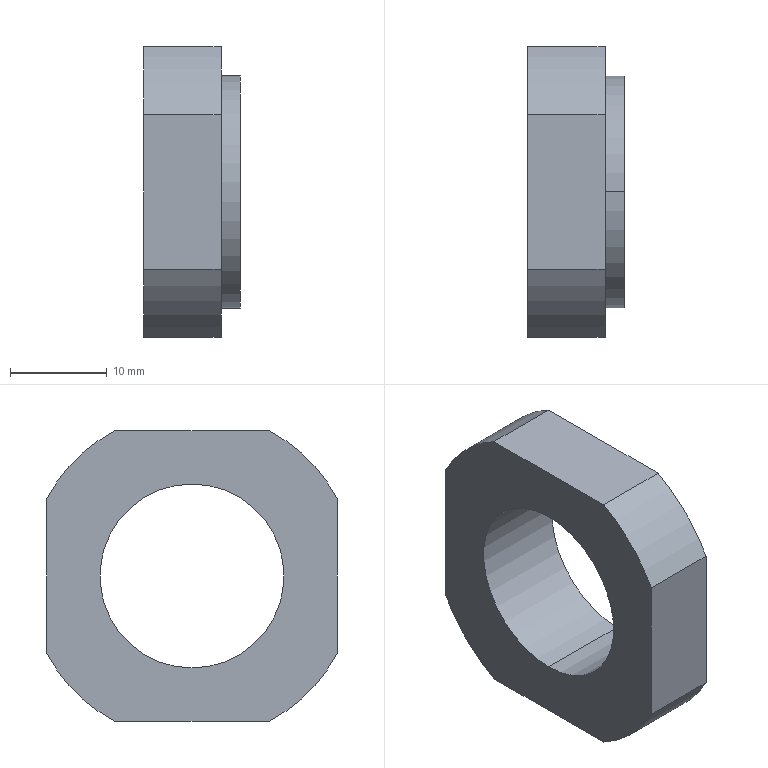Part | STEP file | PN_0006 nut | 1 solid | 15 faces | box 10 x 30 x 30 mm | volume 4642 mm3 | cylinder 8 | plane 7 | commonest cylinder face diameters 34 x4 19 x2 24 x2
STEP:
#1=CARTESIAN_POINT('',(0.,0.,0.));
#2=DIRECTION('',(0.,0.,1.));
#3=DIRECTION('',(1.,0.,0.));
#4=AXIS2_PLACEMENT_3D('',#1,#2,#3);
#5=CARTESIAN_POINT('',(-10.,0.,-9.5));
#6=VERTEX_POINT('',#5);
#7=CARTESIAN_POINT('',(0.,0.,-9.5));
#8=VERTEX_POINT('',#7);
#9=CARTESIAN_POINT('',(-10.,0.,-9.5));
#10=DIRECTION('',(1.,0.,0.));
#11=VECTOR('',#10,1.);
#12=LINE('',#9,#11);
#13=CARTESIAN_POINT('',(-10.,0.,0.));
#14=DIRECTION('',(1.,0.,0.));
#15=DIRECTION('',(0.,0.,-1.));
#16=AXIS2_PLACEMENT_3D('',#13,#14,#15);
#17=CYLINDRICAL_SURFACE('',#16,9.5);
#18=CARTESIAN_POINT('',(6.283,0.));
#19=DIRECTION('',(0.,1.));
#20=VECTOR('',#19,1.);
#21=LINE('',#18,#20);
#22=(GEOMETRIC_REPRESENTATION_CONTEXT(2)PARAMETRIC_REPRESENTATION_CONTEXT()REPRESENTATION_CONTEXT('',''));
#23=DEFINITIONAL_REPRESENTATION('',(#21),#22);
#24=PCURVE('',#17,#23);
#25=CARTESIAN_POINT('',(-10.,0.,0.));
#26=DIRECTION('',(1.,0.,0.));
#27=DIRECTION('',(0.,0.,-1.));
#28=AXIS2_PLACEMENT_3D('',#25,#26,#27);
#29=CYLINDRICAL_SURFACE('',#28,9.5);
#30=CARTESIAN_POINT('',(0.,0.));
#31=DIRECTION('',(0.,1.));
#32=VECTOR('',#31,1.);
#33=LINE('',#30,#32);
#34=(GEOMETRIC_REPRESENTATION_CONTEXT(2)PARAMETRIC_REPRESENTATION_CONTEXT()REPRESENTATION_CONTEXT('',''));
#35=DEFINITIONAL_REPRESENTATION('',(#33),#34);
#36=PCURVE('',#29,#35);
#37=SURFACE_CURVE('',#12,(#24,#36),.PCURVE_S1.);
#38=EDGE_CURVE('',#6,#8,#37,.T.);
#39=ORIENTED_EDGE('',*,*,#38,.T.);
#40=CARTESIAN_POINT('',(0.,0.,9.5));
#41=VERTEX_POINT('',#40);
#42=CARTESIAN_POINT('',(0.,0.,0.));
#43=DIRECTION('',(1.,0.,0.));
#44=DIRECTION('',(0.,0.,-1.));
#45=AXIS2_PLACEMENT_3D('',#42,#43,#44);
#46=CIRCLE('',#45,9.5);
#47=CARTESIAN_POINT('',(0.,10.));
#48=DIRECTION('',(1.,0.));
#49=VECTOR('',#48,1.);
#50=LINE('',#47,#49);
#51=(GEOMETRIC_REPRESENTATION_CONTEXT(2)PARAMETRIC_REPRESENTATION_CONTEXT()REPRESENTATION_CONTEXT('',''));
#52=DEFINITIONAL_REPRESENTATION('',(#50),#51);
#53=PCURVE('',#17,#52);
#54=CARTESIAN_POINT('',(0.,0.,0.));
#55=DIRECTION('',(1.,0.,0.));
#56=DIRECTION('',(0.,0.,-1.));
#57=AXIS2_PLACEMENT_3D('',#54,#55,#56);
#58=PLANE('',#57);
#59=CARTESIAN_POINT('',(0.,0.));
#60=DIRECTION('',(1.,0.));
#61=AXIS2_PLACEMENT_2D('',#59,#60);
#62=CIRCLE('',#61,9.5);
#63=(GEOMETRIC_REPRESENTATION_CONTEXT(2)PARAMETRIC_REPRESENTATION_CONTEXT()REPRESENTATION_CONTEXT('',''));
#64=DEFINITIONAL_REPRESENTATION('',(#62),#63);
#65=PCURVE('',#58,#64);
#66=SURFACE_CURVE('',#46,(#53,#65),.PCURVE_S1.);
#67=EDGE_CURVE('',#41,#8,#66,.T.);
#68=ORIENTED_EDGE('',*,*,#67,.F.);
#69=CARTESIAN_POINT('',(-10.,0.,9.5));
#70=VERTEX_POINT('',#69);
#71=CARTESIAN_POINT('',(-10.,0.,9.5));
#72=DIRECTION('',(1.,0.,0.));
#73=VECTOR('',#72,1.);
#74=LINE('',#71,#73);
#75=CARTESIAN_POINT('',(3.142,0.));
#76=DIRECTION('',(0.,1.));
#77=VECTOR('',#76,1.);
#78=LINE('',#75,#77);
#79=(GEOMETRIC_REPRESENTATION_CONTEXT(2)PARAMETRIC_REPRESENTATION_CONTEXT()REPRESENTATION_CONTEXT('',''));
#80=DEFINITIONAL_REPRESENTATION('',(#78),#79);
#81=PCURVE('',#17,#80);
#82=CARTESIAN_POINT('',(3.142,0.));
#83=DIRECTION('',(0.,1.));
#84=VECTOR('',#83,1.);
#85=LINE('',#82,#84);
#86=(GEOMETRIC_REPRESENTATION_CONTEXT(2)PARAMETRIC_REPRESENTATION_CONTEXT()REPRESENTATION_CONTEXT('',''));
#87=DEFINITIONAL_REPRESENTATION('',(#85),#86);
#88=PCURVE('',#29,#87);
#89=SURFACE_CURVE('',#74,(#81,#88),.PCURVE_S1.);
#90=EDGE_CURVE('',#70,#41,#89,.T.);
#91=ORIENTED_EDGE('',*,*,#90,.F.);
#92=CARTESIAN_POINT('',(-10.,0.,0.));
#93=DIRECTION('',(1.,0.,0.));
#94=DIRECTION('',(0.,0.,-1.));
#95=AXIS2_PLACEMENT_3D('',#92,#93,#94);
#96=CIRCLE('',#95,9.5);
#97=CARTESIAN_POINT('',(0.,0.));
#98=DIRECTION('',(1.,0.));
#99=VECTOR('',#98,1.);
#100=LINE('',#97,#99);
#101=(GEOMETRIC_REPRESENTATION_CONTEXT(2)PARAMETRIC_REPRESENTATION_CONTEXT()REPRESENTATION_CONTEXT('',''));
#102=DEFINITIONAL_REPRESENTATION('',(#100),#101);
#103=PCURVE('',#17,#102);
#104=CARTESIAN_POINT('',(-10.,17.,0.));
#105=DIRECTION('',(-1.,0.,0.));
#106=DIRECTION('',(0.,0.,1.));
#107=AXIS2_PLACEMENT_3D('',#104,#105,#106);
#108=PLANE('',#107);
#109=CARTESIAN_POINT('',(-9.5,-17.));
#110=CARTESIAN_POINT('',(-9.5,-0.5455));
#111=CARTESIAN_POINT('',(4.75,-8.773));
#112=CARTESIAN_POINT('',(19.,-17.));
#113=CARTESIAN_POINT('',(4.75,-25.227));
#114=CARTESIAN_POINT('',(-9.5,-33.454));
#115=CARTESIAN_POINT('',(-9.5,-17.));
#116=(BOUNDED_CURVE()B_SPLINE_CURVE(2,(#109,#110,#111,#112,#113,#114,#115),.UNSPECIFIED.,.T.,.F.)B_SPLINE_CURVE_WITH_KNOTS((1,2,2,2,2,1),(-2.094,0.,2.094,4.189,6.283,8.378),.UNSPECIFIED.)CURVE()GEOMETRIC_REPRESENTATION_ITEM()RATIONAL_B_SPLINE_CURVE((1.,0.5,1.,0.5,1.,0.5,1.))REPRESENTATION_ITEM(''));
#117=(GEOMETRIC_REPRESENTATION_CONTEXT(2)PARAMETRIC_REPRESENTATION_CONTEXT()REPRESENTATION_CONTEXT('',''));
#118=DEFINITIONAL_REPRESENTATION('',(#116),#117);
#119=PCURVE('',#108,#118);
#120=SURFACE_CURVE('',#96,(#103,#119),.PCURVE_S1.);
#121=EDGE_CURVE('',#70,#6,#120,.T.);
#122=ORIENTED_EDGE('',*,*,#121,.T.);
#123=EDGE_LOOP('',(#39,#68,#91,#122));
#124=FACE_BOUND('',#123,.F.);
#125=ADVANCED_FACE('',(#124),#17,.F.);
#126=CARTESIAN_POINT('',(-2.,0.,-12.));
#127=VERTEX_POINT('',#126);
#128=CARTESIAN_POINT('',(-2.,0.,12.));
#129=VERTEX_POINT('',#128);
#130=CARTESIAN_POINT('',(-2.,0.,0.));
#131=DIRECTION('',(1.,0.,0.));
#132=DIRECTION('',(0.,0.,-1.));
#133=AXIS2_PLACEMENT_3D('',#130,#131,#132);
#134=CIRCLE('',#133,12.);
#135=CARTESIAN_POINT('',(0.,0.,0.));
#136=DIRECTION('',(1.,0.,0.));
#137=DIRECTION('',(0.,0.,-1.));
#138=AXIS2_PLACEMENT_3D('',#135,#136,#137);
#139=CYLINDRICAL_SURFACE('',#138,12.);
#140=CARTESIAN_POINT('',(0.,-2.));
#141=DIRECTION('',(1.,0.));
#142=VECTOR('',#141,1.);
#143=LINE('',#140,#142);
#144=(GEOMETRIC_REPRESENTATION_CONTEXT(2)PARAMETRIC_REPRESENTATION_CONTEXT()REPRESENTATION_CONTEXT('',''));
#145=DEFINITIONAL_REPRESENTATION('',(#143),#144);
#146=PCURVE('',#139,#145);
#147=CARTESIAN_POINT('',(-2.,12.,0.));
#148=DIRECTION('',(1.,0.,0.));
#149=DIRECTION('',(0.,0.,-1.));
#150=AXIS2_PLACEMENT_3D('',#147,#148,#149);
#151=PLANE('',#150);
#152=CARTESIAN_POINT('',(0.,-12.));
#153=DIRECTION('',(1.,0.));
#154=AXIS2_PLACEMENT_2D('',#152,#153);
#155=CIRCLE('',#154,12.);
#156=(GEOMETRIC_REPRESENTATION_CONTEXT(2)PARAMETRIC_REPRESENTATION_CONTEXT()REPRESENTATION_CONTEXT('',''));
#157=DEFINITIONAL_REPRESENTATION('',(#155),#156);
#158=PCURVE('',#151,#157);
#159=SURFACE_CURVE('',#134,(#146,#158),.PCURVE_S1.);
#160=EDGE_CURVE('',#127,#129,#159,.T.);
#161=ORIENTED_EDGE('',*,*,#160,.T.);
#162=CARTESIAN_POINT('',(0.,0.,12.));
#163=VERTEX_POINT('',#162);
#164=CARTESIAN_POINT('',(0.,0.,12.));
#165=DIRECTION('',(1.,0.,0.));
#166=VECTOR('',#165,1.);
#167=LINE('',#164,#166);
#168=CARTESIAN_POINT('',(3.142,0.));
#169=DIRECTION('',(0.,1.));
#170=VECTOR('',#169,1.);
#171=LINE('',#168,#170);
#172=(GEOMETRIC_REPRESENTATION_CONTEXT(2)PARAMETRIC_REPRESENTATION_CONTEXT()REPRESENTATION_CONTEXT('',''));
#173=DEFINITIONAL_REPRESENTATION('',(#171),#172);
#174=PCURVE('',#139,#173);
#175=CARTESIAN_POINT('',(0.,0.,0.));
#176=DIRECTION('',(1.,0.,0.));
#177=DIRECTION('',(0.,0.,-1.));
#178=AXIS2_PLACEMENT_3D('',#175,#176,#177);
#179=CYLINDRICAL_SURFACE('',#178,12.);
#180=CARTESIAN_POINT('',(3.142,0.));
#181=DIRECTION('',(0.,1.));
#182=VECTOR('',#181,1.);
#183=LINE('',#180,#182);
#184=(GEOMETRIC_REPRESENTATION_CONTEXT(2)PARAMETRIC_REPRESENTATION_CONTEXT()REPRESENTATION_CONTEXT('',''));
#185=DEFINITIONAL_REPRESENTATION('',(#183),#184);
#186=PCURVE('',#179,#185);
#187=SURFACE_CURVE('',#167,(#174,#186),.PCURVE_S1.);
#188=EDGE_CURVE('',#129,#163,#187,.T.);
#189=ORIENTED_EDGE('',*,*,#188,.T.);
#190=CARTESIAN_POINT('',(0.,0.,-12.));
#191=VERTEX_POINT('',#190);
#192=CARTESIAN_POINT('',(0.,0.,0.));
#193=DIRECTION('',(1.,0.,0.));
#194=DIRECTION('',(0.,0.,-1.));
#195=AXIS2_PLACEMENT_3D('',#192,#193,#194);
#196=CIRCLE('',#195,12.);
#197=CARTESIAN_POINT('',(0.,0.));
#198=DIRECTION('',(1.,0.));
#199=VECTOR('',#198,1.);
#200=LINE('',#197,#199);
#201=(GEOMETRIC_REPRESENTATION_CONTEXT(2)PARAMETRIC_REPRESENTATION_CONTEXT()REPRESENTATION_CONTEXT('',''));
#202=DEFINITIONAL_REPRESENTATION('',(#200),#201);
#203=PCURVE('',#139,#202);
#204=CARTESIAN_POINT('',(0.,0.));
#205=DIRECTION('',(1.,0.));
#206=AXIS2_PLACEMENT_2D('',#204,#205);
#207=CIRCLE('',#206,12.);
#208=(GEOMETRIC_REPRESENTATION_CONTEXT(2)PARAMETRIC_REPRESENTATION_CONTEXT()REPRESENTATION_CONTEXT('',''));
#209=DEFINITIONAL_REPRESENTATION('',(#207),#208);
#210=PCURVE('',#58,#209);
#211=SURFACE_CURVE('',#196,(#203,#210),.PCURVE_S1.);
#212=EDGE_CURVE('',#191,#163,#211,.T.);
#213=ORIENTED_EDGE('',*,*,#212,.F.);
#214=CARTESIAN_POINT('',(0.,0.,-12.));
#215=DIRECTION('',(1.,0.,0.));
#216=VECTOR('',#215,1.);
#217=LINE('',#214,#216);
#218=CARTESIAN_POINT('',(0.,0.));
#219=DIRECTION('',(0.,1.));
#220=VECTOR('',#219,1.);
#221=LINE('',#218,#220);
#222=(GEOMETRIC_REPRESENTATION_CONTEXT(2)PARAMETRIC_REPRESENTATION_CONTEXT()REPRESENTATION_CONTEXT('',''));
#223=DEFINITIONAL_REPRESENTATION('',(#221),#222);
#224=PCURVE('',#139,#223);
#225=CARTESIAN_POINT('',(6.283,0.));
#226=DIRECTION('',(0.,1.));
#227=VECTOR('',#226,1.);
#228=LINE('',#225,#227);
#229=(GEOMETRIC_REPRESENTATION_CONTEXT(2)PARAMETRIC_REPRESENTATION_CONTEXT()REPRESENTATION_CONTEXT('',''));
#230=DEFINITIONAL_REPRESENTATION('',(#228),#229);
#231=PCURVE('',#179,#230);
#232=SURFACE_CURVE('',#217,(#224,#231),.PCURVE_S1.);
#233=EDGE_CURVE('',#127,#191,#232,.T.);
#234=ORIENTED_EDGE('',*,*,#233,.F.);
#235=EDGE_LOOP('',(#161,#189,#213,#234));
#236=FACE_BOUND('',#235,.T.);
#237=ADVANCED_FACE('',(#236),#139,.T.);
#238=CARTESIAN_POINT('',(-2.,8.,15.));
#239=VERTEX_POINT('',#238);
#240=CARTESIAN_POINT('',(-10.,8.,15.));
#241=VERTEX_POINT('',#240);
#242=CARTESIAN_POINT('',(0.,8.,15.));
#243=DIRECTION('',(-1.,0.,0.));
#244=VECTOR('',#243,1.);
#245=LINE('',#242,#244);
#246=CARTESIAN_POINT('',(0.,0.,0.));
#247=DIRECTION('',(1.,0.,0.));
#248=DIRECTION('',(0.,0.,-1.));
#249=AXIS2_PLACEMENT_3D('',#246,#247,#248);
#250=CYLINDRICAL_SURFACE('',#249,17.);
#251=CARTESIAN_POINT('',(2.652,0.));
#252=DIRECTION('',(0.,-1.));
#253=VECTOR('',#252,1.);
#254=LINE('',#251,#253);
#255=(GEOMETRIC_REPRESENTATION_CONTEXT(2)PARAMETRIC_REPRESENTATION_CONTEXT()REPRESENTATION_CONTEXT('',''));
#256=DEFINITIONAL_REPRESENTATION('',(#254),#255);
#257=PCURVE('',#250,#256);
#258=CARTESIAN_POINT('',(0.,17.205,15.));
#259=DIRECTION('',(0.,0.,-1.));
#260=DIRECTION('',(0.,1.,0.));
#261=AXIS2_PLACEMENT_3D('',#258,#259,#260);
#262=PLANE('',#261);
#263=CARTESIAN_POINT('',(-9.205,0.));
#264=DIRECTION('',(0.,-1.));
#265=VECTOR('',#264,1.);
#266=LINE('',#263,#265);
#267=(GEOMETRIC_REPRESENTATION_CONTEXT(2)PARAMETRIC_REPRESENTATION_CONTEXT()REPRESENTATION_CONTEXT('',''));
#268=DEFINITIONAL_REPRESENTATION('',(#266),#267);
#269=PCURVE('',#262,#268);
#270=SURFACE_CURVE('',#245,(#257,#269),.PCURVE_S1.);
#271=EDGE_CURVE('',#239,#241,#270,.T.);
#272=ORIENTED_EDGE('',*,*,#271,.F.);
#273=CARTESIAN_POINT('',(-2.,15.,8.));
#274=VERTEX_POINT('',#273);
#275=CARTESIAN_POINT('',(-2.,0.,0.));
#276=DIRECTION('',(1.,0.,0.));
#277=DIRECTION('',(0.,0.,-1.));
#278=AXIS2_PLACEMENT_3D('',#275,#276,#277);
#279=CIRCLE('',#278,17.);
#280=CARTESIAN_POINT('',(0.,-2.));
#281=DIRECTION('',(1.,0.));
#282=VECTOR('',#281,1.);
#283=LINE('',#280,#282);
#284=(GEOMETRIC_REPRESENTATION_CONTEXT(2)PARAMETRIC_REPRESENTATION_CONTEXT()REPRESENTATION_CONTEXT('',''));
#285=DEFINITIONAL_REPRESENTATION('',(#283),#284);
#286=PCURVE('',#250,#285);
#287=CARTESIAN_POINT('',(0.,-12.));
#288=DIRECTION('',(1.,0.));
#289=AXIS2_PLACEMENT_2D('',#287,#288);
#290=CIRCLE('',#289,17.);
#291=(GEOMETRIC_REPRESENTATION_CONTEXT(2)PARAMETRIC_REPRESENTATION_CONTEXT()REPRESENTATION_CONTEXT('',''));
#292=DEFINITIONAL_REPRESENTATION('',(#290),#291);
#293=PCURVE('',#151,#292);
#294=SURFACE_CURVE('',#279,(#286,#293),.PCURVE_S1.);
#295=EDGE_CURVE('',#274,#239,#294,.T.);
#296=ORIENTED_EDGE('',*,*,#295,.F.);
#297=CARTESIAN_POINT('',(-10.,15.,8.));
#298=VERTEX_POINT('',#297);
#299=CARTESIAN_POINT('',(0.,15.,8.));
#300=DIRECTION('',(1.,0.,0.));
#301=VECTOR('',#300,1.);
#302=LINE('',#299,#301);
#303=CARTESIAN_POINT('',(2.061,0.));
#304=DIRECTION('',(0.,1.));
#305=VECTOR('',#304,1.);
#306=LINE('',#303,#305);
#307=(GEOMETRIC_REPRESENTATION_CONTEXT(2)PARAMETRIC_REPRESENTATION_CONTEXT()REPRESENTATION_CONTEXT('',''));
#308=DEFINITIONAL_REPRESENTATION('',(#306),#307);
#309=PCURVE('',#250,#308);
#310=CARTESIAN_POINT('',(0.,15.,-20.296));
#311=DIRECTION('',(0.,-1.,0.));
#312=DIRECTION('',(0.,0.,-1.));
#313=AXIS2_PLACEMENT_3D('',#310,#311,#312);
#314=PLANE('',#313);
#315=CARTESIAN_POINT('',(-28.296,0.));
#316=DIRECTION('',(0.,1.));
#317=VECTOR('',#316,1.);
#318=LINE('',#315,#317);
#319=(GEOMETRIC_REPRESENTATION_CONTEXT(2)PARAMETRIC_REPRESENTATION_CONTEXT()REPRESENTATION_CONTEXT('',''));
#320=DEFINITIONAL_REPRESENTATION('',(#318),#319);
#321=PCURVE('',#314,#320);
#322=SURFACE_CURVE('',#302,(#309,#321),.PCURVE_S1.);
#323=EDGE_CURVE('',#298,#274,#322,.T.);
#324=ORIENTED_EDGE('',*,*,#323,.F.);
#325=CARTESIAN_POINT('',(-10.,0.,0.));
#326=DIRECTION('',(1.,0.,0.));
#327=DIRECTION('',(0.,0.,-1.));
#328=AXIS2_PLACEMENT_3D('',#325,#326,#327);
#329=CIRCLE('',#328,17.);
#330=CARTESIAN_POINT('',(0.,-10.));
#331=DIRECTION('',(1.,0.));
#332=VECTOR('',#331,1.);
#333=LINE('',#330,#332);
#334=(GEOMETRIC_REPRESENTATION_CONTEXT(2)PARAMETRIC_REPRESENTATION_CONTEXT()REPRESENTATION_CONTEXT('',''));
#335=DEFINITIONAL_REPRESENTATION('',(#333),#334);
#336=PCURVE('',#250,#335);
#337=CARTESIAN_POINT('',(-17.,-17.));
#338=CARTESIAN_POINT('',(-17.,12.445));
#339=CARTESIAN_POINT('',(8.5,-2.278));
#340=CARTESIAN_POINT('',(34.,-17.));
#341=CARTESIAN_POINT('',(8.5,-31.722));
#342=CARTESIAN_POINT('',(-17.,-46.445));
#343=CARTESIAN_POINT('',(-17.,-17.));
#344=(BOUNDED_CURVE()B_SPLINE_CURVE(2,(#337,#338,#339,#340,#341,#342,#343),.UNSPECIFIED.,.T.,.F.)B_SPLINE_CURVE_WITH_KNOTS((1,2,2,2,2,1),(-2.094,0.,2.094,4.189,6.283,8.378),.UNSPECIFIED.)CURVE()GEOMETRIC_REPRESENTATION_ITEM()RATIONAL_B_SPLINE_CURVE((1.,0.5,1.,0.5,1.,0.5,1.))REPRESENTATION_ITEM(''));
#345=(GEOMETRIC_REPRESENTATION_CONTEXT(2)PARAMETRIC_REPRESENTATION_CONTEXT()REPRESENTATION_CONTEXT('',''));
#346=DEFINITIONAL_REPRESENTATION('',(#344),#345);
#347=PCURVE('',#108,#346);
#348=SURFACE_CURVE('',#329,(#336,#347),.PCURVE_S1.);
#349=EDGE_CURVE('',#298,#241,#348,.T.);
#350=ORIENTED_EDGE('',*,*,#349,.T.);
#351=EDGE_LOOP('',(#272,#296,#324,#350));
#352=FACE_BOUND('',#351,.T.);
#353=ADVANCED_FACE('',(#352),#250,.T.);
#354=CARTESIAN_POINT('',(-2.,-8.,-15.));
#355=VERTEX_POINT('',#354);
#356=CARTESIAN_POINT('',(-10.,-8.,-15.));
#357=VERTEX_POINT('',#356);
#358=CARTESIAN_POINT('',(0.,-8.,-15.));
#359=DIRECTION('',(-1.,0.,0.));
#360=VECTOR('',#359,1.);
#361=LINE('',#358,#360);
#362=CARTESIAN_POINT('',(0.,0.,0.));
#363=DIRECTION('',(1.,0.,0.));
#364=DIRECTION('',(0.,0.,-1.));
#365=AXIS2_PLACEMENT_3D('',#362,#363,#364);
#366=CYLINDRICAL_SURFACE('',#365,17.);
#367=CARTESIAN_POINT('',(5.793,0.));
#368=DIRECTION('',(0.,-1.));
#369=VECTOR('',#368,1.);
#370=LINE('',#367,#369);
#371=(GEOMETRIC_REPRESENTATION_CONTEXT(2)PARAMETRIC_REPRESENTATION_CONTEXT()REPRESENTATION_CONTEXT('',''));
#372=DEFINITIONAL_REPRESENTATION('',(#370),#371);
#373=PCURVE('',#366,#372);
#374=CARTESIAN_POINT('',(0.,17.205,-15.));
#375=DIRECTION('',(0.,0.,1.));
#376=DIRECTION('',(0.,-1.,0.));
#377=AXIS2_PLACEMENT_3D('',#374,#375,#376);
#378=PLANE('',#377);
#379=CARTESIAN_POINT('',(25.205,0.));
#380=DIRECTION('',(0.,-1.));
#381=VECTOR('',#380,1.);
#382=LINE('',#379,#381);
#383=(GEOMETRIC_REPRESENTATION_CONTEXT(2)PARAMETRIC_REPRESENTATION_CONTEXT()REPRESENTATION_CONTEXT('',''));
#384=DEFINITIONAL_REPRESENTATION('',(#382),#383);
#385=PCURVE('',#378,#384);
#386=SURFACE_CURVE('',#361,(#373,#385),.PCURVE_S1.);
#387=EDGE_CURVE('',#355,#357,#386,.T.);
#388=ORIENTED_EDGE('',*,*,#387,.F.);
#389=CARTESIAN_POINT('',(-2.,-15.,-8.));
#390=VERTEX_POINT('',#389);
#391=CARTESIAN_POINT('',(-2.,0.,0.));
#392=DIRECTION('',(1.,0.,0.));
#393=DIRECTION('',(0.,0.,-1.));
#394=AXIS2_PLACEMENT_3D('',#391,#392,#393);
#395=CIRCLE('',#394,17.);
#396=CARTESIAN_POINT('',(0.,-2.));
#397=DIRECTION('',(1.,0.));
#398=VECTOR('',#397,1.);
#399=LINE('',#396,#398);
#400=(GEOMETRIC_REPRESENTATION_CONTEXT(2)PARAMETRIC_REPRESENTATION_CONTEXT()REPRESENTATION_CONTEXT('',''));
#401=DEFINITIONAL_REPRESENTATION('',(#399),#400);
#402=PCURVE('',#366,#401);
#403=CARTESIAN_POINT('',(0.,-12.));
#404=DIRECTION('',(1.,0.));
#405=AXIS2_PLACEMENT_2D('',#403,#404);
#406=CIRCLE('',#405,17.);
#407=(GEOMETRIC_REPRESENTATION_CONTEXT(2)PARAMETRIC_REPRESENTATION_CONTEXT()REPRESENTATION_CONTEXT('',''));
#408=DEFINITIONAL_REPRESENTATION('',(#406),#407);
#409=PCURVE('',#151,#408);
#410=SURFACE_CURVE('',#395,(#402,#409),.PCURVE_S1.);
#411=EDGE_CURVE('',#390,#355,#410,.T.);
#412=ORIENTED_EDGE('',*,*,#411,.F.);
#413=CARTESIAN_POINT('',(-10.,-15.,-8.));
#414=VERTEX_POINT('',#413);
#415=CARTESIAN_POINT('',(0.,-15.,-8.));
#416=DIRECTION('',(1.,0.,0.));
#417=VECTOR('',#416,1.);
#418=LINE('',#415,#417);
#419=CARTESIAN_POINT('',(5.202,0.));
#420=DIRECTION('',(0.,1.));
#421=VECTOR('',#420,1.);
#422=LINE('',#419,#421);
#423=(GEOMETRIC_REPRESENTATION_CONTEXT(2)PARAMETRIC_REPRESENTATION_CONTEXT()REPRESENTATION_CONTEXT('',''));
#424=DEFINITIONAL_REPRESENTATION('',(#422),#423);
#425=PCURVE('',#366,#424);
#426=CARTESIAN_POINT('',(0.,-15.,-20.296));
#427=DIRECTION('',(0.,1.,0.));
#428=DIRECTION('',(0.,0.,1.));
#429=AXIS2_PLACEMENT_3D('',#426,#427,#428);
#430=PLANE('',#429);
#431=CARTESIAN_POINT('',(12.296,0.));
#432=DIRECTION('',(0.,1.));
#433=VECTOR('',#432,1.);
#434=LINE('',#431,#433);
#435=(GEOMETRIC_REPRESENTATION_CONTEXT(2)PARAMETRIC_REPRESENTATION_CONTEXT()REPRESENTATION_CONTEXT('',''));
#436=DEFINITIONAL_REPRESENTATION('',(#434),#435);
#437=PCURVE('',#430,#436);
#438=SURFACE_CURVE('',#418,(#425,#437),.PCURVE_S1.);
#439=EDGE_CURVE('',#414,#390,#438,.T.);
#440=ORIENTED_EDGE('',*,*,#439,.F.);
#441=CARTESIAN_POINT('',(-10.,0.,0.));
#442=DIRECTION('',(1.,0.,0.));
#443=DIRECTION('',(0.,0.,-1.));
#444=AXIS2_PLACEMENT_3D('',#441,#442,#443);
#445=CIRCLE('',#444,17.);
#446=CARTESIAN_POINT('',(0.,-10.));
#447=DIRECTION('',(1.,0.));
#448=VECTOR('',#447,1.);
#449=LINE('',#446,#448);
#450=(GEOMETRIC_REPRESENTATION_CONTEXT(2)PARAMETRIC_REPRESENTATION_CONTEXT()REPRESENTATION_CONTEXT('',''));
#451=DEFINITIONAL_REPRESENTATION('',(#449),#450);
#452=PCURVE('',#366,#451);
#453=CARTESIAN_POINT('',(-17.,-17.));
#454=CARTESIAN_POINT('',(-17.,12.445));
#455=CARTESIAN_POINT('',(8.5,-2.278));
#456=CARTESIAN_POINT('',(34.,-17.));
#457=CARTESIAN_POINT('',(8.5,-31.722));
#458=CARTESIAN_POINT('',(-17.,-46.445));
#459=CARTESIAN_POINT('',(-17.,-17.));
#460=(BOUNDED_CURVE()B_SPLINE_CURVE(2,(#453,#454,#455,#456,#457,#458,#459),.UNSPECIFIED.,.T.,.F.)B_SPLINE_CURVE_WITH_KNOTS((1,2,2,2,2,1),(-2.094,0.,2.094,4.189,6.283,8.378),.UNSPECIFIED.)CURVE()GEOMETRIC_REPRESENTATION_ITEM()RATIONAL_B_SPLINE_CURVE((1.,0.5,1.,0.5,1.,0.5,1.))REPRESENTATION_ITEM(''));
#461=(GEOMETRIC_REPRESENTATION_CONTEXT(2)PARAMETRIC_REPRESENTATION_CONTEXT()REPRESENTATION_CONTEXT('',''));
#462=DEFINITIONAL_REPRESENTATION('',(#460),#461);
#463=PCURVE('',#108,#462);
#464=SURFACE_CURVE('',#445,(#452,#463),.PCURVE_S1.);
#465=EDGE_CURVE('',#414,#357,#464,.T.);
#466=ORIENTED_EDGE('',*,*,#465,.T.);
#467=EDGE_LOOP('',(#388,#412,#440,#466));
#468=FACE_BOUND('',#467,.T.);
#469=ADVANCED_FACE('',(#468),#366,.T.);
#470=CARTESIAN_POINT('',(-10.,-8.,15.));
#471=VERTEX_POINT('',#470);
#472=CARTESIAN_POINT('',(-2.,-8.,15.));
#473=VERTEX_POINT('',#472);
#474=CARTESIAN_POINT('',(0.,-8.,15.));
#475=DIRECTION('',(1.,0.,0.));
#476=VECTOR('',#475,1.);
#477=LINE('',#474,#476);
#478=CARTESIAN_POINT('',(0.,0.,0.));
#479=DIRECTION('',(1.,0.,0.));
#480=DIRECTION('',(0.,0.,-1.));
#481=AXIS2_PLACEMENT_3D('',#478,#479,#480);
#482=CYLINDRICAL_SURFACE('',#481,17.);
#483=CARTESIAN_POINT('',(3.632,0.));
#484=DIRECTION('',(0.,1.));
#485=VECTOR('',#484,1.);
#486=LINE('',#483,#485);
#487=(GEOMETRIC_REPRESENTATION_CONTEXT(2)PARAMETRIC_REPRESENTATION_CONTEXT()REPRESENTATION_CONTEXT('',''));
#488=DEFINITIONAL_REPRESENTATION('',(#486),#487);
#489=PCURVE('',#482,#488);
#490=CARTESIAN_POINT('',(-25.205,0.));
#491=DIRECTION('',(0.,1.));
#492=VECTOR('',#491,1.);
#493=LINE('',#490,#492);
#494=(GEOMETRIC_REPRESENTATION_CONTEXT(2)PARAMETRIC_REPRESENTATION_CONTEXT()REPRESENTATION_CONTEXT('',''));
#495=DEFINITIONAL_REPRESENTATION('',(#493),#494);
#496=PCURVE('',#262,#495);
#497=SURFACE_CURVE('',#477,(#489,#496),.PCURVE_S1.);
#498=EDGE_CURVE('',#471,#473,#497,.T.);
#499=ORIENTED_EDGE('',*,*,#498,.F.);
#500=CARTESIAN_POINT('',(-10.,-15.,8.));
#501=VERTEX_POINT('',#500);
#502=CARTESIAN_POINT('',(-10.,0.,0.));
#503=DIRECTION('',(1.,0.,0.));
#504=DIRECTION('',(0.,0.,-1.));
#505=AXIS2_PLACEMENT_3D('',#502,#503,#504);
#506=CIRCLE('',#505,17.);
#507=CARTESIAN_POINT('',(0.,-10.));
#508=DIRECTION('',(1.,0.));
#509=VECTOR('',#508,1.);
#510=LINE('',#507,#509);
#511=(GEOMETRIC_REPRESENTATION_CONTEXT(2)PARAMETRIC_REPRESENTATION_CONTEXT()REPRESENTATION_CONTEXT('',''));
#512=DEFINITIONAL_REPRESENTATION('',(#510),#511);
#513=PCURVE('',#482,#512);
#514=CARTESIAN_POINT('',(-17.,-17.));
#515=CARTESIAN_POINT('',(-17.,12.445));
#516=CARTESIAN_POINT('',(8.5,-2.278));
#517=CARTESIAN_POINT('',(34.,-17.));
#518=CARTESIAN_POINT('',(8.5,-31.722));
#519=CARTESIAN_POINT('',(-17.,-46.445));
#520=CARTESIAN_POINT('',(-17.,-17.));
#521=(BOUNDED_CURVE()B_SPLINE_CURVE(2,(#514,#515,#516,#517,#518,#519,#520),.UNSPECIFIED.,.T.,.F.)B_SPLINE_CURVE_WITH_KNOTS((1,2,2,2,2,1),(-2.094,0.,2.094,4.189,6.283,8.378),.UNSPECIFIED.)CURVE()GEOMETRIC_REPRESENTATION_ITEM()RATIONAL_B_SPLINE_CURVE((1.,0.5,1.,0.5,1.,0.5,1.))REPRESENTATION_ITEM(''));
#522=(GEOMETRIC_REPRESENTATION_CONTEXT(2)PARAMETRIC_REPRESENTATION_CONTEXT()REPRESENTATION_CONTEXT('',''));
#523=DEFINITIONAL_REPRESENTATION('',(#521),#522);
#524=PCURVE('',#108,#523);
#525=SURFACE_CURVE('',#506,(#513,#524),.PCURVE_S1.);
#526=EDGE_CURVE('',#471,#501,#525,.T.);
#527=ORIENTED_EDGE('',*,*,#526,.T.);
#528=CARTESIAN_POINT('',(-2.,-15.,8.));
#529=VERTEX_POINT('',#528);
#530=CARTESIAN_POINT('',(0.,-15.,8.));
#531=DIRECTION('',(-1.,0.,0.));
#532=VECTOR('',#531,1.);
#533=LINE('',#530,#532);
#534=CARTESIAN_POINT('',(4.222,0.));
#535=DIRECTION('',(0.,-1.));
#536=VECTOR('',#535,1.);
#537=LINE('',#534,#536);
#538=(GEOMETRIC_REPRESENTATION_CONTEXT(2)PARAMETRIC_REPRESENTATION_CONTEXT()REPRESENTATION_CONTEXT('',''));
#539=DEFINITIONAL_REPRESENTATION('',(#537),#538);
#540=PCURVE('',#482,#539);
#541=CARTESIAN_POINT('',(28.296,0.));
#542=DIRECTION('',(0.,-1.));
#543=VECTOR('',#542,1.);
#544=LINE('',#541,#543);
#545=(GEOMETRIC_REPRESENTATION_CONTEXT(2)PARAMETRIC_REPRESENTATION_CONTEXT()REPRESENTATION_CONTEXT('',''));
#546=DEFINITIONAL_REPRESENTATION('',(#544),#545);
#547=PCURVE('',#430,#546);
#548=SURFACE_CURVE('',#533,(#540,#547),.PCURVE_S1.);
#549=EDGE_CURVE('',#529,#501,#548,.T.);
#550=ORIENTED_EDGE('',*,*,#549,.F.);
#551=CARTESIAN_POINT('',(-2.,0.,0.));
#552=DIRECTION('',(1.,0.,0.));
#553=DIRECTION('',(0.,0.,-1.));
#554=AXIS2_PLACEMENT_3D('',#551,#552,#553);
#555=CIRCLE('',#554,17.);
#556=CARTESIAN_POINT('',(0.,-2.));
#557=DIRECTION('',(1.,0.));
#558=VECTOR('',#557,1.);
#559=LINE('',#556,#558);
#560=(GEOMETRIC_REPRESENTATION_CONTEXT(2)PARAMETRIC_REPRESENTATION_CONTEXT()REPRESENTATION_CONTEXT('',''));
#561=DEFINITIONAL_REPRESENTATION('',(#559),#560);
#562=PCURVE('',#482,#561);
#563=CARTESIAN_POINT('',(0.,-12.));
#564=DIRECTION('',(1.,0.));
#565=AXIS2_PLACEMENT_2D('',#563,#564);
#566=CIRCLE('',#565,17.);
#567=(GEOMETRIC_REPRESENTATION_CONTEXT(2)PARAMETRIC_REPRESENTATION_CONTEXT()REPRESENTATION_CONTEXT('',''));
#568=DEFINITIONAL_REPRESENTATION('',(#566),#567);
#569=PCURVE('',#151,#568);
#570=SURFACE_CURVE('',#555,(#562,#569),.PCURVE_S1.);
#571=EDGE_CURVE('',#473,#529,#570,.T.);
#572=ORIENTED_EDGE('',*,*,#571,.F.);
#573=EDGE_LOOP('',(#499,#527,#550,#572));
#574=FACE_BOUND('',#573,.T.);
#575=ADVANCED_FACE('',(#574),#482,.T.);
#576=CARTESIAN_POINT('',(0.,0.,0.));
#577=DIRECTION('',(1.,0.,0.));
#578=DIRECTION('',(0.,0.,-1.));
#579=AXIS2_PLACEMENT_3D('',#576,#577,#578);
#580=CIRCLE('',#579,9.5);
#581=CARTESIAN_POINT('',(0.,0.));
#582=DIRECTION('',(1.,0.));
#583=AXIS2_PLACEMENT_2D('',#581,#582);
#584=CIRCLE('',#583,9.5);
#585=(GEOMETRIC_REPRESENTATION_CONTEXT(2)PARAMETRIC_REPRESENTATION_CONTEXT()REPRESENTATION_CONTEXT('',''));
#586=DEFINITIONAL_REPRESENTATION('',(#584),#585);
#587=PCURVE('',#58,#586);
#588=CARTESIAN_POINT('',(0.,10.));
#589=DIRECTION('',(1.,0.));
#590=VECTOR('',#589,1.);
#591=LINE('',#588,#590);
#592=(GEOMETRIC_REPRESENTATION_CONTEXT(2)PARAMETRIC_REPRESENTATION_CONTEXT()REPRESENTATION_CONTEXT('',''));
#593=DEFINITIONAL_REPRESENTATION('',(#591),#592);
#594=PCURVE('',#29,#593);
#595=SURFACE_CURVE('',#580,(#587,#594),.PCURVE_S1.);
#596=EDGE_CURVE('',#8,#41,#595,.T.);
#597=ORIENTED_EDGE('',*,*,#596,.F.);
#598=ORIENTED_EDGE('',*,*,#67,.F.);
#599=EDGE_LOOP('',(#597,#598));
#600=FACE_BOUND('',#599,.T.);
#601=ORIENTED_EDGE('',*,*,#212,.T.);
#602=CARTESIAN_POINT('',(0.,0.,0.));
#603=DIRECTION('',(1.,0.,0.));
#604=DIRECTION('',(0.,0.,-1.));
#605=AXIS2_PLACEMENT_3D('',#602,#603,#604);
#606=CIRCLE('',#605,12.);
#607=CARTESIAN_POINT('',(0.,0.));
#608=DIRECTION('',(1.,0.));
#609=AXIS2_PLACEMENT_2D('',#607,#608);
#610=CIRCLE('',#609,12.);
#611=(GEOMETRIC_REPRESENTATION_CONTEXT(2)PARAMETRIC_REPRESENTATION_CONTEXT()REPRESENTATION_CONTEXT('',''));
#612=DEFINITIONAL_REPRESENTATION('',(#610),#611);
#613=PCURVE('',#58,#612);
#614=CARTESIAN_POINT('',(0.,0.));
#615=DIRECTION('',(1.,0.));
#616=VECTOR('',#615,1.);
#617=LINE('',#614,#616);
#618=(GEOMETRIC_REPRESENTATION_CONTEXT(2)PARAMETRIC_REPRESENTATION_CONTEXT()REPRESENTATION_CONTEXT('',''));
#619=DEFINITIONAL_REPRESENTATION('',(#617),#618);
#620=PCURVE('',#179,#619);
#621=SURFACE_CURVE('',#606,(#613,#620),.PCURVE_S1.);
#622=EDGE_CURVE('',#163,#191,#621,.T.);
#623=ORIENTED_EDGE('',*,*,#622,.T.);
#624=EDGE_LOOP('',(#601,#623));
#625=FACE_BOUND('',#624,.T.);
#626=ADVANCED_FACE('',(#600,#625),#58,.T.);
#627=ORIENTED_EDGE('',*,*,#188,.F.);
#628=CARTESIAN_POINT('',(-2.,0.,0.));
#629=DIRECTION('',(1.,0.,0.));
#630=DIRECTION('',(0.,0.,-1.));
#631=AXIS2_PLACEMENT_3D('',#628,#629,#630);
#632=CIRCLE('',#631,12.);
#633=CARTESIAN_POINT('',(0.,-2.));
#634=DIRECTION('',(1.,0.));
#635=VECTOR('',#634,1.);
#636=LINE('',#633,#635);
#637=(GEOMETRIC_REPRESENTATION_CONTEXT(2)PARAMETRIC_REPRESENTATION_CONTEXT()REPRESENTATION_CONTEXT('',''));
#638=DEFINITIONAL_REPRESENTATION('',(#636),#637);
#639=PCURVE('',#179,#638);
#640=CARTESIAN_POINT('',(0.,-12.));
#641=DIRECTION('',(1.,0.));
#642=AXIS2_PLACEMENT_2D('',#640,#641);
#643=CIRCLE('',#642,12.);
#644=(GEOMETRIC_REPRESENTATION_CONTEXT(2)PARAMETRIC_REPRESENTATION_CONTEXT()REPRESENTATION_CONTEXT('',''));
#645=DEFINITIONAL_REPRESENTATION('',(#643),#644);
#646=PCURVE('',#151,#645);
#647=SURFACE_CURVE('',#632,(#639,#646),.PCURVE_S1.);
#648=EDGE_CURVE('',#129,#127,#647,.T.);
#649=ORIENTED_EDGE('',*,*,#648,.T.);
#650=ORIENTED_EDGE('',*,*,#233,.T.);
#651=ORIENTED_EDGE('',*,*,#622,.F.);
#652=EDGE_LOOP('',(#627,#649,#650,#651));
#653=FACE_BOUND('',#652,.T.);
#654=ADVANCED_FACE('',(#653),#179,.T.);
#655=CARTESIAN_POINT('',(-2.,12.,15.));
#656=DIRECTION('',(0.,1.,0.));
#657=VECTOR('',#656,1.);
#658=LINE('',#655,#657);
#659=CARTESIAN_POINT('',(-15.,0.));
#660=DIRECTION('',(0.,1.));
#661=VECTOR('',#660,1.);
#662=LINE('',#659,#661);
#663=(GEOMETRIC_REPRESENTATION_CONTEXT(2)PARAMETRIC_REPRESENTATION_CONTEXT()REPRESENTATION_CONTEXT('',''));
#664=DEFINITIONAL_REPRESENTATION('',(#662),#663);
#665=PCURVE('',#151,#664);
#666=CARTESIAN_POINT('',(-5.205,-2.));
#667=DIRECTION('',(1.,0.));
#668=VECTOR('',#667,1.);
#669=LINE('',#666,#668);
#670=(GEOMETRIC_REPRESENTATION_CONTEXT(2)PARAMETRIC_REPRESENTATION_CONTEXT()REPRESENTATION_CONTEXT('',''));
#671=DEFINITIONAL_REPRESENTATION('',(#669),#670);
#672=PCURVE('',#262,#671);
#673=SURFACE_CURVE('',#658,(#665,#672),.PCURVE_S1.);
#674=EDGE_CURVE('',#473,#239,#673,.T.);
#675=ORIENTED_EDGE('',*,*,#674,.F.);
#676=ORIENTED_EDGE('',*,*,#571,.T.);
#677=CARTESIAN_POINT('',(-2.,-15.,0.));
#678=DIRECTION('',(0.,0.,1.));
#679=VECTOR('',#678,1.);
#680=LINE('',#677,#679);
#681=CARTESIAN_POINT('',(0.,-27.));
#682=DIRECTION('',(-1.,0.));
#683=VECTOR('',#682,1.);
#684=LINE('',#681,#683);
#685=(GEOMETRIC_REPRESENTATION_CONTEXT(2)PARAMETRIC_REPRESENTATION_CONTEXT()REPRESENTATION_CONTEXT('',''));
#686=DEFINITIONAL_REPRESENTATION('',(#684),#685);
#687=PCURVE('',#151,#686);
#688=CARTESIAN_POINT('',(20.296,-2.));
#689=DIRECTION('',(1.,0.));
#690=VECTOR('',#689,1.);
#691=LINE('',#688,#690);
#692=(GEOMETRIC_REPRESENTATION_CONTEXT(2)PARAMETRIC_REPRESENTATION_CONTEXT()REPRESENTATION_CONTEXT('',''));
#693=DEFINITIONAL_REPRESENTATION('',(#691),#692);
#694=PCURVE('',#430,#693);
#695=SURFACE_CURVE('',#680,(#687,#694),.PCURVE_S1.);
#696=EDGE_CURVE('',#390,#529,#695,.T.);
#697=ORIENTED_EDGE('',*,*,#696,.F.);
#698=ORIENTED_EDGE('',*,*,#411,.T.);
#699=CARTESIAN_POINT('',(-2.,8.,-15.));
#700=VERTEX_POINT('',#699);
#701=CARTESIAN_POINT('',(-2.,12.,-15.));
#702=DIRECTION('',(0.,-1.,0.));
#703=VECTOR('',#702,1.);
#704=LINE('',#701,#703);
#705=CARTESIAN_POINT('',(15.,0.));
#706=DIRECTION('',(0.,-1.));
#707=VECTOR('',#706,1.);
#708=LINE('',#705,#707);
#709=(GEOMETRIC_REPRESENTATION_CONTEXT(2)PARAMETRIC_REPRESENTATION_CONTEXT()REPRESENTATION_CONTEXT('',''));
#710=DEFINITIONAL_REPRESENTATION('',(#708),#709);
#711=PCURVE('',#151,#710);
#712=CARTESIAN_POINT('',(5.205,-2.));
#713=DIRECTION('',(1.,0.));
#714=VECTOR('',#713,1.);
#715=LINE('',#712,#714);
#716=(GEOMETRIC_REPRESENTATION_CONTEXT(2)PARAMETRIC_REPRESENTATION_CONTEXT()REPRESENTATION_CONTEXT('',''));
#717=DEFINITIONAL_REPRESENTATION('',(#715),#716);
#718=PCURVE('',#378,#717);
#719=SURFACE_CURVE('',#704,(#711,#718),.PCURVE_S1.);
#720=EDGE_CURVE('',#700,#355,#719,.T.);
#721=ORIENTED_EDGE('',*,*,#720,.F.);
#722=CARTESIAN_POINT('',(-2.,15.,-8.));
#723=VERTEX_POINT('',#722);
#724=CARTESIAN_POINT('',(-2.,0.,0.));
#725=DIRECTION('',(1.,0.,0.));
#726=DIRECTION('',(0.,0.,-1.));
#727=AXIS2_PLACEMENT_3D('',#724,#725,#726);
#728=CIRCLE('',#727,17.);
#729=CARTESIAN_POINT('',(0.,-12.));
#730=DIRECTION('',(1.,0.));
#731=AXIS2_PLACEMENT_2D('',#729,#730);
#732=CIRCLE('',#731,17.);
#733=(GEOMETRIC_REPRESENTATION_CONTEXT(2)PARAMETRIC_REPRESENTATION_CONTEXT()REPRESENTATION_CONTEXT('',''));
#734=DEFINITIONAL_REPRESENTATION('',(#732),#733);
#735=PCURVE('',#151,#734);
#736=CARTESIAN_POINT('',(0.,0.,0.));
#737=DIRECTION('',(1.,0.,0.));
#738=DIRECTION('',(0.,0.,-1.));
#739=AXIS2_PLACEMENT_3D('',#736,#737,#738);
#740=CYLINDRICAL_SURFACE('',#739,17.);
#741=CARTESIAN_POINT('',(0.,-2.));
#742=DIRECTION('',(1.,0.));
#743=VECTOR('',#742,1.);
#744=LINE('',#741,#743);
#745=(GEOMETRIC_REPRESENTATION_CONTEXT(2)PARAMETRIC_REPRESENTATION_CONTEXT()REPRESENTATION_CONTEXT('',''));
#746=DEFINITIONAL_REPRESENTATION('',(#744),#745);
#747=PCURVE('',#740,#746);
#748=SURFACE_CURVE('',#728,(#735,#747),.PCURVE_S1.);
#749=EDGE_CURVE('',#700,#723,#748,.T.);
#750=ORIENTED_EDGE('',*,*,#749,.T.);
#751=CARTESIAN_POINT('',(-2.,15.,0.));
#752=DIRECTION('',(0.,0.,-1.));
#753=VECTOR('',#752,1.);
#754=LINE('',#751,#753);
#755=CARTESIAN_POINT('',(0.,3.));
#756=DIRECTION('',(1.,0.));
#757=VECTOR('',#756,1.);
#758=LINE('',#755,#757);
#759=(GEOMETRIC_REPRESENTATION_CONTEXT(2)PARAMETRIC_REPRESENTATION_CONTEXT()REPRESENTATION_CONTEXT('',''));
#760=DEFINITIONAL_REPRESENTATION('',(#758),#759);
#761=PCURVE('',#151,#760);
#762=CARTESIAN_POINT('',(-20.296,-2.));
#763=DIRECTION('',(1.,0.));
#764=VECTOR('',#763,1.);
#765=LINE('',#762,#764);
#766=(GEOMETRIC_REPRESENTATION_CONTEXT(2)PARAMETRIC_REPRESENTATION_CONTEXT()REPRESENTATION_CONTEXT('',''));
#767=DEFINITIONAL_REPRESENTATION('',(#765),#766);
#768=PCURVE('',#314,#767);
#769=SURFACE_CURVE('',#754,(#761,#768),.PCURVE_S1.);
#770=EDGE_CURVE('',#274,#723,#769,.T.);
#771=ORIENTED_EDGE('',*,*,#770,.F.);
#772=ORIENTED_EDGE('',*,*,#295,.T.);
#773=EDGE_LOOP('',(#675,#676,#697,#698,#721,#750,#771,#772));
#774=FACE_BOUND('',#773,.T.);
#775=ORIENTED_EDGE('',*,*,#160,.F.);
#776=ORIENTED_EDGE('',*,*,#648,.F.);
#777=EDGE_LOOP('',(#775,#776));
#778=FACE_BOUND('',#777,.T.);
#779=ADVANCED_FACE('',(#774,#778),#151,.T.);
#780=CARTESIAN_POINT('',(-10.,8.,-15.));
#781=VERTEX_POINT('',#780);
#782=CARTESIAN_POINT('',(0.,8.,-15.));
#783=DIRECTION('',(1.,0.,0.));
#784=VECTOR('',#783,1.);
#785=LINE('',#782,#784);
#786=CARTESIAN_POINT('',(0.49,0.));
#787=DIRECTION('',(0.,1.));
#788=VECTOR('',#787,1.);
#789=LINE('',#786,#788);
#790=(GEOMETRIC_REPRESENTATION_CONTEXT(2)PARAMETRIC_REPRESENTATION_CONTEXT()REPRESENTATION_CONTEXT('',''));
#791=DEFINITIONAL_REPRESENTATION('',(#789),#790);
#792=PCURVE('',#740,#791);
#793=CARTESIAN_POINT('',(9.205,0.));
#794=DIRECTION('',(0.,1.));
#795=VECTOR('',#794,1.);
#796=LINE('',#793,#795);
#797=(GEOMETRIC_REPRESENTATION_CONTEXT(2)PARAMETRIC_REPRESENTATION_CONTEXT()REPRESENTATION_CONTEXT('',''));
#798=DEFINITIONAL_REPRESENTATION('',(#796),#797);
#799=PCURVE('',#378,#798);
#800=SURFACE_CURVE('',#785,(#792,#799),.PCURVE_S1.);
#801=EDGE_CURVE('',#781,#700,#800,.T.);
#802=ORIENTED_EDGE('',*,*,#801,.F.);
#803=CARTESIAN_POINT('',(-10.,15.,-8.));
#804=VERTEX_POINT('',#803);
#805=CARTESIAN_POINT('',(-10.,0.,0.));
#806=DIRECTION('',(1.,0.,0.));
#807=DIRECTION('',(0.,0.,-1.));
#808=AXIS2_PLACEMENT_3D('',#805,#806,#807);
#809=CIRCLE('',#808,17.);
#810=CARTESIAN_POINT('',(0.,-10.));
#811=DIRECTION('',(1.,0.));
#812=VECTOR('',#811,1.);
#813=LINE('',#810,#812);
#814=(GEOMETRIC_REPRESENTATION_CONTEXT(2)PARAMETRIC_REPRESENTATION_CONTEXT()REPRESENTATION_CONTEXT('',''));
#815=DEFINITIONAL_REPRESENTATION('',(#813),#814);
#816=PCURVE('',#740,#815);
#817=CARTESIAN_POINT('',(-17.,-17.));
#818=CARTESIAN_POINT('',(-17.,12.445));
#819=CARTESIAN_POINT('',(8.5,-2.278));
#820=CARTESIAN_POINT('',(34.,-17.));
#821=CARTESIAN_POINT('',(8.5,-31.722));
#822=CARTESIAN_POINT('',(-17.,-46.445));
#823=CARTESIAN_POINT('',(-17.,-17.));
#824=(BOUNDED_CURVE()B_SPLINE_CURVE(2,(#817,#818,#819,#820,#821,#822,#823),.UNSPECIFIED.,.T.,.F.)B_SPLINE_CURVE_WITH_KNOTS((1,2,2,2,2,1),(-2.094,0.,2.094,4.189,6.283,8.378),.UNSPECIFIED.)CURVE()GEOMETRIC_REPRESENTATION_ITEM()RATIONAL_B_SPLINE_CURVE((1.,0.5,1.,0.5,1.,0.5,1.))REPRESENTATION_ITEM(''));
#825=(GEOMETRIC_REPRESENTATION_CONTEXT(2)PARAMETRIC_REPRESENTATION_CONTEXT()REPRESENTATION_CONTEXT('',''));
#826=DEFINITIONAL_REPRESENTATION('',(#824),#825);
#827=PCURVE('',#108,#826);
#828=SURFACE_CURVE('',#809,(#816,#827),.PCURVE_S1.);
#829=EDGE_CURVE('',#781,#804,#828,.T.);
#830=ORIENTED_EDGE('',*,*,#829,.T.);
#831=CARTESIAN_POINT('',(0.,15.,-8.));
#832=DIRECTION('',(-1.,0.,0.));
#833=VECTOR('',#832,1.);
#834=LINE('',#831,#833);
#835=CARTESIAN_POINT('',(1.081,0.));
#836=DIRECTION('',(0.,-1.));
#837=VECTOR('',#836,1.);
#838=LINE('',#835,#837);
#839=(GEOMETRIC_REPRESENTATION_CONTEXT(2)PARAMETRIC_REPRESENTATION_CONTEXT()REPRESENTATION_CONTEXT('',''));
#840=DEFINITIONAL_REPRESENTATION('',(#838),#839);
#841=PCURVE('',#740,#840);
#842=CARTESIAN_POINT('',(-12.296,0.));
#843=DIRECTION('',(0.,-1.));
#844=VECTOR('',#843,1.);
#845=LINE('',#842,#844);
#846=(GEOMETRIC_REPRESENTATION_CONTEXT(2)PARAMETRIC_REPRESENTATION_CONTEXT()REPRESENTATION_CONTEXT('',''));
#847=DEFINITIONAL_REPRESENTATION('',(#845),#846);
#848=PCURVE('',#314,#847);
#849=SURFACE_CURVE('',#834,(#841,#848),.PCURVE_S1.);
#850=EDGE_CURVE('',#723,#804,#849,.T.);
#851=ORIENTED_EDGE('',*,*,#850,.F.);
#852=ORIENTED_EDGE('',*,*,#749,.F.);
#853=EDGE_LOOP('',(#802,#830,#851,#852));
#854=FACE_BOUND('',#853,.T.);
#855=ADVANCED_FACE('',(#854),#740,.T.);
#856=CARTESIAN_POINT('',(-10.,17.,15.));
#857=DIRECTION('',(0.,-1.,0.));
#858=VECTOR('',#857,1.);
#859=LINE('',#856,#858);
#860=CARTESIAN_POINT('',(15.,0.));
#861=DIRECTION('',(0.,-1.));
#862=VECTOR('',#861,1.);
#863=LINE('',#860,#862);
#864=(GEOMETRIC_REPRESENTATION_CONTEXT(2)PARAMETRIC_REPRESENTATION_CONTEXT()REPRESENTATION_CONTEXT('',''));
#865=DEFINITIONAL_REPRESENTATION('',(#863),#864);
#866=PCURVE('',#108,#865);
#867=CARTESIAN_POINT('',(-0.2052,-10.));
#868=DIRECTION('',(-1.,0.));
#869=VECTOR('',#868,1.);
#870=LINE('',#867,#869);
#871=(GEOMETRIC_REPRESENTATION_CONTEXT(2)PARAMETRIC_REPRESENTATION_CONTEXT()REPRESENTATION_CONTEXT('',''));
#872=DEFINITIONAL_REPRESENTATION('',(#870),#871);
#873=PCURVE('',#262,#872);
#874=SURFACE_CURVE('',#859,(#866,#873),.PCURVE_S1.);
#875=EDGE_CURVE('',#241,#471,#874,.T.);
#876=ORIENTED_EDGE('',*,*,#875,.F.);
#877=ORIENTED_EDGE('',*,*,#349,.F.);
#878=CARTESIAN_POINT('',(-10.,15.,0.));
#879=DIRECTION('',(0.,0.,1.));
#880=VECTOR('',#879,1.);
#881=LINE('',#878,#880);
#882=CARTESIAN_POINT('',(0.,-2.));
#883=DIRECTION('',(1.,0.));
#884=VECTOR('',#883,1.);
#885=LINE('',#882,#884);
#886=(GEOMETRIC_REPRESENTATION_CONTEXT(2)PARAMETRIC_REPRESENTATION_CONTEXT()REPRESENTATION_CONTEXT('',''));
#887=DEFINITIONAL_REPRESENTATION('',(#885),#886);
#888=PCURVE('',#108,#887);
#889=CARTESIAN_POINT('',(-20.296,-10.));
#890=DIRECTION('',(-1.,0.));
#891=VECTOR('',#890,1.);
#892=LINE('',#889,#891);
#893=(GEOMETRIC_REPRESENTATION_CONTEXT(2)PARAMETRIC_REPRESENTATION_CONTEXT()REPRESENTATION_CONTEXT('',''));
#894=DEFINITIONAL_REPRESENTATION('',(#892),#893);
#895=PCURVE('',#314,#894);
#896=SURFACE_CURVE('',#881,(#888,#895),.PCURVE_S1.);
#897=EDGE_CURVE('',#804,#298,#896,.T.);
#898=ORIENTED_EDGE('',*,*,#897,.F.);
#899=ORIENTED_EDGE('',*,*,#829,.F.);
#900=CARTESIAN_POINT('',(-10.,17.,-15.));
#901=DIRECTION('',(0.,1.,0.));
#902=VECTOR('',#901,1.);
#903=LINE('',#900,#902);
#904=CARTESIAN_POINT('',(-15.,0.));
#905=DIRECTION('',(0.,1.));
#906=VECTOR('',#905,1.);
#907=LINE('',#904,#906);
#908=(GEOMETRIC_REPRESENTATION_CONTEXT(2)PARAMETRIC_REPRESENTATION_CONTEXT()REPRESENTATION_CONTEXT('',''));
#909=DEFINITIONAL_REPRESENTATION('',(#907),#908);
#910=PCURVE('',#108,#909);
#911=CARTESIAN_POINT('',(0.2052,-10.));
#912=DIRECTION('',(-1.,0.));
#913=VECTOR('',#912,1.);
#914=LINE('',#911,#913);
#915=(GEOMETRIC_REPRESENTATION_CONTEXT(2)PARAMETRIC_REPRESENTATION_CONTEXT()REPRESENTATION_CONTEXT('',''));
#916=DEFINITIONAL_REPRESENTATION('',(#914),#915);
#917=PCURVE('',#378,#916);
#918=SURFACE_CURVE('',#903,(#910,#917),.PCURVE_S1.);
#919=EDGE_CURVE('',#357,#781,#918,.T.);
#920=ORIENTED_EDGE('',*,*,#919,.F.);
#921=ORIENTED_EDGE('',*,*,#465,.F.);
#922=CARTESIAN_POINT('',(-10.,-15.,0.));
#923=DIRECTION('',(0.,0.,-1.));
#924=VECTOR('',#923,1.);
#925=LINE('',#922,#924);
#926=CARTESIAN_POINT('',(0.,-32.));
#927=DIRECTION('',(-1.,0.));
#928=VECTOR('',#927,1.);
#929=LINE('',#926,#928);
#930=(GEOMETRIC_REPRESENTATION_CONTEXT(2)PARAMETRIC_REPRESENTATION_CONTEXT()REPRESENTATION_CONTEXT('',''));
#931=DEFINITIONAL_REPRESENTATION('',(#929),#930);
#932=PCURVE('',#108,#931);
#933=CARTESIAN_POINT('',(20.296,-10.));
#934=DIRECTION('',(-1.,0.));
#935=VECTOR('',#934,1.);
#936=LINE('',#933,#935);
#937=(GEOMETRIC_REPRESENTATION_CONTEXT(2)PARAMETRIC_REPRESENTATION_CONTEXT()REPRESENTATION_CONTEXT('',''));
#938=DEFINITIONAL_REPRESENTATION('',(#936),#937);
#939=PCURVE('',#430,#938);
#940=SURFACE_CURVE('',#925,(#932,#939),.PCURVE_S1.);
#941=EDGE_CURVE('',#501,#414,#940,.T.);
#942=ORIENTED_EDGE('',*,*,#941,.F.);
#943=ORIENTED_EDGE('',*,*,#526,.F.);
#944=EDGE_LOOP('',(#876,#877,#898,#899,#920,#921,#942,#943));
#945=FACE_BOUND('',#944,.T.);
#946=CARTESIAN_POINT('',(-10.,0.,0.));
#947=DIRECTION('',(1.,0.,0.));
#948=DIRECTION('',(0.,0.,-1.));
#949=AXIS2_PLACEMENT_3D('',#946,#947,#948);
#950=CIRCLE('',#949,9.5);
#951=CARTESIAN_POINT('',(-9.5,-17.));
#952=CARTESIAN_POINT('',(-9.5,-0.5455));
#953=CARTESIAN_POINT('',(4.75,-8.773));
#954=CARTESIAN_POINT('',(19.,-17.));
#955=CARTESIAN_POINT('',(4.75,-25.227));
#956=CARTESIAN_POINT('',(-9.5,-33.454));
#957=CARTESIAN_POINT('',(-9.5,-17.));
#958=(BOUNDED_CURVE()B_SPLINE_CURVE(2,(#951,#952,#953,#954,#955,#956,#957),.UNSPECIFIED.,.T.,.F.)B_SPLINE_CURVE_WITH_KNOTS((1,2,2,2,2,1),(-2.094,0.,2.094,4.189,6.283,8.378),.UNSPECIFIED.)CURVE()GEOMETRIC_REPRESENTATION_ITEM()RATIONAL_B_SPLINE_CURVE((1.,0.5,1.,0.5,1.,0.5,1.))REPRESENTATION_ITEM(''));
#959=(GEOMETRIC_REPRESENTATION_CONTEXT(2)PARAMETRIC_REPRESENTATION_CONTEXT()REPRESENTATION_CONTEXT('',''));
#960=DEFINITIONAL_REPRESENTATION('',(#958),#959);
#961=PCURVE('',#108,#960);
#962=CARTESIAN_POINT('',(0.,0.));
#963=DIRECTION('',(1.,0.));
#964=VECTOR('',#963,1.);
#965=LINE('',#962,#964);
#966=(GEOMETRIC_REPRESENTATION_CONTEXT(2)PARAMETRIC_REPRESENTATION_CONTEXT()REPRESENTATION_CONTEXT('',''));
#967=DEFINITIONAL_REPRESENTATION('',(#965),#966);
#968=PCURVE('',#29,#967);
#969=SURFACE_CURVE('',#950,(#961,#968),.PCURVE_S1.);
#970=EDGE_CURVE('',#6,#70,#969,.T.);
#971=ORIENTED_EDGE('',*,*,#970,.T.);
#972=ORIENTED_EDGE('',*,*,#121,.T.);
#973=EDGE_LOOP('',(#971,#972));
#974=FACE_BOUND('',#973,.T.);
#975=ADVANCED_FACE('',(#945,#974),#108,.T.);
#976=ORIENTED_EDGE('',*,*,#596,.F.);
#977=ORIENTED_EDGE('',*,*,#38,.F.);
#978=ORIENTED_EDGE('',*,*,#970,.T.);
#979=ORIENTED_EDGE('',*,*,#90,.T.);
#980=EDGE_LOOP('',(#976,#977,#978,#979));
#981=FACE_BOUND('',#980,.F.);
#982=ADVANCED_FACE('',(#981),#29,.F.);
#983=ORIENTED_EDGE('',*,*,#850,.T.);
#984=ORIENTED_EDGE('',*,*,#897,.T.);
#985=ORIENTED_EDGE('',*,*,#323,.T.);
#986=ORIENTED_EDGE('',*,*,#770,.T.);
#987=EDGE_LOOP('',(#983,#984,#985,#986));
#988=FACE_BOUND('',#987,.T.);
#989=ADVANCED_FACE('',(#988),#314,.F.);
#990=ORIENTED_EDGE('',*,*,#549,.T.);
#991=ORIENTED_EDGE('',*,*,#941,.T.);
#992=ORIENTED_EDGE('',*,*,#439,.T.);
#993=ORIENTED_EDGE('',*,*,#696,.T.);
#994=EDGE_LOOP('',(#990,#991,#992,#993));
#995=FACE_BOUND('',#994,.T.);
#996=ADVANCED_FACE('',(#995),#430,.F.);
#997=ORIENTED_EDGE('',*,*,#387,.T.);
#998=ORIENTED_EDGE('',*,*,#919,.T.);
#999=ORIENTED_EDGE('',*,*,#801,.T.);
#1000=ORIENTED_EDGE('',*,*,#720,.T.);
#1001=EDGE_LOOP('',(#997,#998,#999,#1000));
#1002=FACE_BOUND('',#1001,.T.);
#1003=ADVANCED_FACE('',(#1002),#378,.F.);
#1004=ORIENTED_EDGE('',*,*,#271,.T.);
#1005=ORIENTED_EDGE('',*,*,#875,.T.);
#1006=ORIENTED_EDGE('',*,*,#498,.T.);
#1007=ORIENTED_EDGE('',*,*,#674,.T.);
#1008=EDGE_LOOP('',(#1004,#1005,#1006,#1007));
#1009=FACE_BOUND('',#1008,.T.);
#1010=ADVANCED_FACE('',(#1009),#262,.F.);
#1011=CLOSED_SHELL('',(#125,#237,#353,#469,#575,#626,#654,#779,#855,#975,#982,#989,#996,#1003,#1010));
#1012=MANIFOLD_SOLID_BREP('',#1011);
#1013=(LENGTH_UNIT()NAMED_UNIT(*)SI_UNIT(.MILLI.,.METRE.));
#1014=UNCERTAINTY_MEASURE_WITH_UNIT(LENGTH_MEASURE(0.0000001),#1013,'','');
#1015=(NAMED_UNIT(*)PLANE_ANGLE_UNIT()SI_UNIT($,.RADIAN.));
#1016=(NAMED_UNIT(*)SI_UNIT($,.STERADIAN.)SOLID_ANGLE_UNIT());
#1017=(GEOMETRIC_REPRESENTATION_CONTEXT(3)GLOBAL_UNCERTAINTY_ASSIGNED_CONTEXT((#1014))GLOBAL_UNIT_ASSIGNED_CONTEXT((#1013,#1015,#1016))REPRESENTATION_CONTEXT('',''));
#1018=ADVANCED_BREP_SHAPE_REPRESENTATION('',(#4,#1012),#1017);